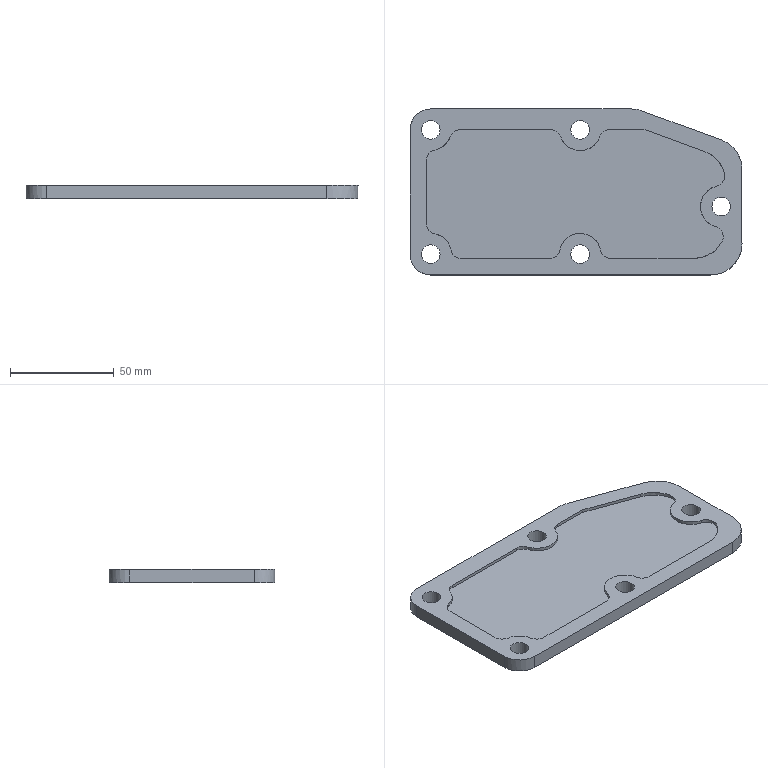Part | SolidWorks | features BaseBody 1 | 1 solid | 69 faces | box 160 x 80 x 6.5 mm | volume 65692 mm3 | cylinder 55 | plane 14 | commonest cylinder face diameters 9 x30 10 x11 20 x9 30 x4 29.999 x1